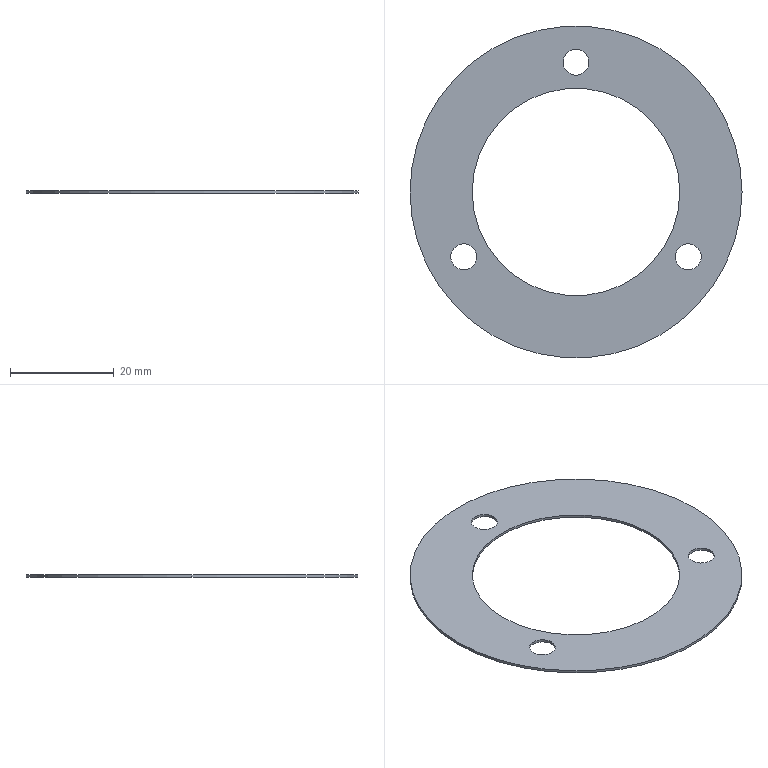Part | SolidWorks | features Extrusion 1, ICE 1 | 1 solid | 12 faces | box 64 x 64 x 0.5 mm | volume 950.724 mm3 | cylinder 10 | plane 2 | commonest cylinder face diameters 5 x6 40 x2 64 x2
STEP:
#1=CARTESIAN_POINT('',(-2.5,25.,0.));
#2=VERTEX_POINT('',#1);
#3=CARTESIAN_POINT('',(2.5,25.,0.));
#4=VERTEX_POINT('',#3);
#5=CARTESIAN_POINT('',(0.,25.,0.));
#6=DIRECTION('',(0.,0.,1.));
#7=DIRECTION('',(1.,0.,0.));
#8=AXIS2_PLACEMENT_3D('',#5,#6,#7);
#9=CIRCLE('',#8,2.5);
#10=EDGE_CURVE('',#2,#4,#9,.T.);
#11=ORIENTED_EDGE('',*,*,#10,.F.);
#12=CARTESIAN_POINT('',(-2.5,25.,0.5));
#13=VERTEX_POINT('',#12);
#14=CARTESIAN_POINT('',(-2.5,25.,0.));
#15=DIRECTION('',(0.,0.,1.));
#16=VECTOR('',#15,1000.);
#17=LINE('',#14,#16);
#18=EDGE_CURVE('',#2,#13,#17,.T.);
#19=ORIENTED_EDGE('',*,*,#18,.T.);
#20=CARTESIAN_POINT('',(2.5,25.,0.5));
#21=VERTEX_POINT('',#20);
#22=CARTESIAN_POINT('',(0.,25.,0.5));
#23=DIRECTION('',(0.,0.,1.));
#24=DIRECTION('',(1.,0.,0.));
#25=AXIS2_PLACEMENT_3D('',#22,#23,#24);
#26=CIRCLE('',#25,2.5);
#27=EDGE_CURVE('',#13,#21,#26,.T.);
#28=ORIENTED_EDGE('',*,*,#27,.T.);
#29=CARTESIAN_POINT('',(2.5,25.,0.));
#30=DIRECTION('',(0.,0.,1.));
#31=VECTOR('',#30,1000.);
#32=LINE('',#29,#31);
#33=EDGE_CURVE('',#4,#21,#32,.T.);
#34=ORIENTED_EDGE('',*,*,#33,.F.);
#35=EDGE_LOOP('',(#11,#19,#28,#34));
#36=FACE_OUTER_BOUND('',#35,.T.);
#37=CARTESIAN_POINT('',(0.,25.,0.));
#38=DIRECTION('',(0.,0.,1.));
#39=DIRECTION('',(1.,0.,0.));
#40=AXIS2_PLACEMENT_3D('',#37,#38,#39);
#41=CYLINDRICAL_SURFACE('',#40,2.5);
#42=ADVANCED_FACE('',(#36),#41,.F.);
#43=CARTESIAN_POINT('',(19.151,-12.5,0.));
#44=VERTEX_POINT('',#43);
#45=CARTESIAN_POINT('',(24.151,-12.5,0.));
#46=VERTEX_POINT('',#45);
#47=CARTESIAN_POINT('',(21.651,-12.5,0.));
#48=DIRECTION('',(0.,0.,1.));
#49=DIRECTION('',(1.,0.,0.));
#50=AXIS2_PLACEMENT_3D('',#47,#48,#49);
#51=CIRCLE('',#50,2.5);
#52=EDGE_CURVE('',#44,#46,#51,.T.);
#53=ORIENTED_EDGE('',*,*,#52,.F.);
#54=CARTESIAN_POINT('',(19.151,-12.5,0.5));
#55=VERTEX_POINT('',#54);
#56=CARTESIAN_POINT('',(19.151,-12.5,0.));
#57=DIRECTION('',(0.,0.,1.));
#58=VECTOR('',#57,1000.);
#59=LINE('',#56,#58);
#60=EDGE_CURVE('',#44,#55,#59,.T.);
#61=ORIENTED_EDGE('',*,*,#60,.T.);
#62=CARTESIAN_POINT('',(24.151,-12.5,0.5));
#63=VERTEX_POINT('',#62);
#64=CARTESIAN_POINT('',(21.651,-12.5,0.5));
#65=DIRECTION('',(0.,0.,1.));
#66=DIRECTION('',(1.,0.,0.));
#67=AXIS2_PLACEMENT_3D('',#64,#65,#66);
#68=CIRCLE('',#67,2.5);
#69=EDGE_CURVE('',#55,#63,#68,.T.);
#70=ORIENTED_EDGE('',*,*,#69,.T.);
#71=CARTESIAN_POINT('',(24.151,-12.5,0.));
#72=DIRECTION('',(0.,0.,1.));
#73=VECTOR('',#72,1000.);
#74=LINE('',#71,#73);
#75=EDGE_CURVE('',#46,#63,#74,.T.);
#76=ORIENTED_EDGE('',*,*,#75,.F.);
#77=EDGE_LOOP('',(#53,#61,#70,#76));
#78=FACE_OUTER_BOUND('',#77,.T.);
#79=CARTESIAN_POINT('',(21.651,-12.5,0.));
#80=DIRECTION('',(0.,0.,1.));
#81=DIRECTION('',(1.,0.,0.));
#82=AXIS2_PLACEMENT_3D('',#79,#80,#81);
#83=CYLINDRICAL_SURFACE('',#82,2.5);
#84=ADVANCED_FACE('',(#78),#83,.F.);
#85=CARTESIAN_POINT('',(-24.151,-12.5,0.));
#86=VERTEX_POINT('',#85);
#87=CARTESIAN_POINT('',(-19.151,-12.5,0.));
#88=VERTEX_POINT('',#87);
#89=CARTESIAN_POINT('',(-21.651,-12.5,0.));
#90=DIRECTION('',(0.,0.,1.));
#91=DIRECTION('',(1.,0.,0.));
#92=AXIS2_PLACEMENT_3D('',#89,#90,#91);
#93=CIRCLE('',#92,2.5);
#94=EDGE_CURVE('',#86,#88,#93,.T.);
#95=ORIENTED_EDGE('',*,*,#94,.F.);
#96=CARTESIAN_POINT('',(-24.151,-12.5,0.5));
#97=VERTEX_POINT('',#96);
#98=CARTESIAN_POINT('',(-24.151,-12.5,0.));
#99=DIRECTION('',(0.,0.,1.));
#100=VECTOR('',#99,1000.);
#101=LINE('',#98,#100);
#102=EDGE_CURVE('',#86,#97,#101,.T.);
#103=ORIENTED_EDGE('',*,*,#102,.T.);
#104=CARTESIAN_POINT('',(-19.151,-12.5,0.5));
#105=VERTEX_POINT('',#104);
#106=CARTESIAN_POINT('',(-21.651,-12.5,0.5));
#107=DIRECTION('',(0.,0.,1.));
#108=DIRECTION('',(1.,0.,0.));
#109=AXIS2_PLACEMENT_3D('',#106,#107,#108);
#110=CIRCLE('',#109,2.5);
#111=EDGE_CURVE('',#97,#105,#110,.T.);
#112=ORIENTED_EDGE('',*,*,#111,.T.);
#113=CARTESIAN_POINT('',(-19.151,-12.5,0.));
#114=DIRECTION('',(0.,0.,1.));
#115=VECTOR('',#114,1000.);
#116=LINE('',#113,#115);
#117=EDGE_CURVE('',#88,#105,#116,.T.);
#118=ORIENTED_EDGE('',*,*,#117,.F.);
#119=EDGE_LOOP('',(#95,#103,#112,#118));
#120=FACE_OUTER_BOUND('',#119,.T.);
#121=CARTESIAN_POINT('',(-21.651,-12.5,0.));
#122=DIRECTION('',(0.,0.,1.));
#123=DIRECTION('',(1.,0.,0.));
#124=AXIS2_PLACEMENT_3D('',#121,#122,#123);
#125=CYLINDRICAL_SURFACE('',#124,2.5);
#126=ADVANCED_FACE('',(#120),#125,.F.);
#127=CARTESIAN_POINT('',(-20.,0.,0.5));
#128=VERTEX_POINT('',#127);
#129=CARTESIAN_POINT('',(20.,0.,0.5));
#130=VERTEX_POINT('',#129);
#131=CARTESIAN_POINT('',(0.,0.,0.5));
#132=DIRECTION('',(0.,0.,1.));
#133=DIRECTION('',(1.,0.,0.));
#134=AXIS2_PLACEMENT_3D('',#131,#132,#133);
#135=CIRCLE('',#134,20.);
#136=EDGE_CURVE('',#128,#130,#135,.T.);
#137=ORIENTED_EDGE('',*,*,#136,.T.);
#138=CARTESIAN_POINT('',(20.,0.,0.));
#139=VERTEX_POINT('',#138);
#140=CARTESIAN_POINT('',(20.,0.,0.5));
#141=DIRECTION('',(0.,0.,-1.));
#142=VECTOR('',#141,1000.);
#143=LINE('',#140,#142);
#144=EDGE_CURVE('',#130,#139,#143,.T.);
#145=ORIENTED_EDGE('',*,*,#144,.T.);
#146=CARTESIAN_POINT('',(-20.,0.,0.));
#147=VERTEX_POINT('',#146);
#148=CARTESIAN_POINT('',(0.,0.,0.));
#149=DIRECTION('',(0.,0.,1.));
#150=DIRECTION('',(1.,0.,0.));
#151=AXIS2_PLACEMENT_3D('',#148,#149,#150);
#152=CIRCLE('',#151,20.);
#153=EDGE_CURVE('',#147,#139,#152,.T.);
#154=ORIENTED_EDGE('',*,*,#153,.F.);
#155=CARTESIAN_POINT('',(-20.,0.,0.5));
#156=DIRECTION('',(0.,0.,-1.));
#157=VECTOR('',#156,1000.);
#158=LINE('',#155,#157);
#159=EDGE_CURVE('',#128,#147,#158,.T.);
#160=ORIENTED_EDGE('',*,*,#159,.F.);
#161=EDGE_LOOP('',(#137,#145,#154,#160));
#162=FACE_OUTER_BOUND('',#161,.T.);
#163=CARTESIAN_POINT('',(0.,0.,0.5));
#164=DIRECTION('',(0.,0.,-1.));
#165=DIRECTION('',(-1.,0.,0.));
#166=AXIS2_PLACEMENT_3D('',#163,#164,#165);
#167=CYLINDRICAL_SURFACE('',#166,20.);
#168=ADVANCED_FACE('',(#162),#167,.F.);
#169=CARTESIAN_POINT('',(32.,0.,0.5));
#170=VERTEX_POINT('',#169);
#171=CARTESIAN_POINT('',(-32.,0.,0.5));
#172=VERTEX_POINT('',#171);
#173=CARTESIAN_POINT('',(0.,0.,0.5));
#174=DIRECTION('',(0.,0.,1.));
#175=DIRECTION('',(1.,0.,0.));
#176=AXIS2_PLACEMENT_3D('',#173,#174,#175);
#177=CIRCLE('',#176,32.);
#178=EDGE_CURVE('',#170,#172,#177,.T.);
#179=ORIENTED_EDGE('',*,*,#178,.F.);
#180=CARTESIAN_POINT('',(32.,0.,0.));
#181=VERTEX_POINT('',#180);
#182=CARTESIAN_POINT('',(32.,0.,0.5));
#183=DIRECTION('',(0.,0.,-1.));
#184=VECTOR('',#183,1000.);
#185=LINE('',#182,#184);
#186=EDGE_CURVE('',#170,#181,#185,.T.);
#187=ORIENTED_EDGE('',*,*,#186,.T.);
#188=CARTESIAN_POINT('',(-32.,0.,0.));
#189=VERTEX_POINT('',#188);
#190=CARTESIAN_POINT('',(0.,0.,0.));
#191=DIRECTION('',(0.,0.,1.));
#192=DIRECTION('',(1.,0.,0.));
#193=AXIS2_PLACEMENT_3D('',#190,#191,#192);
#194=CIRCLE('',#193,32.);
#195=EDGE_CURVE('',#181,#189,#194,.T.);
#196=ORIENTED_EDGE('',*,*,#195,.T.);
#197=CARTESIAN_POINT('',(-32.,0.,0.5));
#198=DIRECTION('',(0.,0.,-1.));
#199=VECTOR('',#198,1000.);
#200=LINE('',#197,#199);
#201=EDGE_CURVE('',#172,#189,#200,.T.);
#202=ORIENTED_EDGE('',*,*,#201,.F.);
#203=EDGE_LOOP('',(#179,#187,#196,#202));
#204=FACE_OUTER_BOUND('',#203,.T.);
#205=CARTESIAN_POINT('',(0.,0.,0.5));
#206=DIRECTION('',(0.,0.,-1.));
#207=DIRECTION('',(-1.,0.,0.));
#208=AXIS2_PLACEMENT_3D('',#205,#206,#207);
#209=CYLINDRICAL_SURFACE('',#208,32.);
#210=ADVANCED_FACE('',(#204),#209,.T.);
#211=CARTESIAN_POINT('',(0.,25.,0.5));
#212=DIRECTION('',(0.,0.,1.));
#213=DIRECTION('',(1.,0.,0.));
#214=AXIS2_PLACEMENT_3D('',#211,#212,#213);
#215=CIRCLE('',#214,2.5);
#216=EDGE_CURVE('',#21,#13,#215,.T.);
#217=ORIENTED_EDGE('',*,*,#216,.F.);
#218=ORIENTED_EDGE('',*,*,#27,.F.);
#219=EDGE_LOOP('',(#217,#218));
#220=FACE_BOUND('',#219,.T.);
#221=CARTESIAN_POINT('',(21.651,-12.5,0.5));
#222=DIRECTION('',(0.,0.,1.));
#223=DIRECTION('',(1.,0.,0.));
#224=AXIS2_PLACEMENT_3D('',#221,#222,#223);
#225=CIRCLE('',#224,2.5);
#226=EDGE_CURVE('',#63,#55,#225,.T.);
#227=ORIENTED_EDGE('',*,*,#226,.F.);
#228=ORIENTED_EDGE('',*,*,#69,.F.);
#229=EDGE_LOOP('',(#227,#228));
#230=FACE_BOUND('',#229,.T.);
#231=CARTESIAN_POINT('',(-21.651,-12.5,0.5));
#232=DIRECTION('',(0.,0.,1.));
#233=DIRECTION('',(1.,0.,0.));
#234=AXIS2_PLACEMENT_3D('',#231,#232,#233);
#235=CIRCLE('',#234,2.5);
#236=EDGE_CURVE('',#105,#97,#235,.T.);
#237=ORIENTED_EDGE('',*,*,#236,.F.);
#238=ORIENTED_EDGE('',*,*,#111,.F.);
#239=EDGE_LOOP('',(#237,#238));
#240=FACE_BOUND('',#239,.T.);
#241=CARTESIAN_POINT('',(0.,0.,0.5));
#242=DIRECTION('',(0.,0.,1.));
#243=DIRECTION('',(1.,0.,0.));
#244=AXIS2_PLACEMENT_3D('',#241,#242,#243);
#245=CIRCLE('',#244,32.);
#246=EDGE_CURVE('',#172,#170,#245,.T.);
#247=ORIENTED_EDGE('',*,*,#246,.T.);
#248=ORIENTED_EDGE('',*,*,#178,.T.);
#249=EDGE_LOOP('',(#247,#248));
#250=FACE_OUTER_BOUND('',#249,.T.);
#251=ORIENTED_EDGE('',*,*,#136,.F.);
#252=CARTESIAN_POINT('',(0.,0.,0.5));
#253=DIRECTION('',(0.,0.,1.));
#254=DIRECTION('',(1.,0.,0.));
#255=AXIS2_PLACEMENT_3D('',#252,#253,#254);
#256=CIRCLE('',#255,20.);
#257=EDGE_CURVE('',#130,#128,#256,.T.);
#258=ORIENTED_EDGE('',*,*,#257,.F.);
#259=EDGE_LOOP('',(#251,#258));
#260=FACE_BOUND('',#259,.T.);
#261=CARTESIAN_POINT('',(0.,0.,0.5));
#262=DIRECTION('',(0.,0.,1.));
#263=DIRECTION('',(1.,0.,0.));
#264=AXIS2_PLACEMENT_3D('',#261,#262,#263);
#265=PLANE('',#264);
#266=ADVANCED_FACE('',(#220,#230,#240,#250,#260),#265,.T.);
#267=CARTESIAN_POINT('',(0.,25.,0.));
#268=DIRECTION('',(0.,0.,1.));
#269=DIRECTION('',(1.,0.,0.));
#270=AXIS2_PLACEMENT_3D('',#267,#268,#269);
#271=CIRCLE('',#270,2.5);
#272=EDGE_CURVE('',#4,#2,#271,.T.);
#273=ORIENTED_EDGE('',*,*,#272,.T.);
#274=ORIENTED_EDGE('',*,*,#10,.T.);
#275=EDGE_LOOP('',(#273,#274));
#276=FACE_BOUND('',#275,.T.);
#277=CARTESIAN_POINT('',(21.651,-12.5,0.));
#278=DIRECTION('',(0.,0.,1.));
#279=DIRECTION('',(1.,0.,0.));
#280=AXIS2_PLACEMENT_3D('',#277,#278,#279);
#281=CIRCLE('',#280,2.5);
#282=EDGE_CURVE('',#46,#44,#281,.T.);
#283=ORIENTED_EDGE('',*,*,#282,.T.);
#284=ORIENTED_EDGE('',*,*,#52,.T.);
#285=EDGE_LOOP('',(#283,#284));
#286=FACE_BOUND('',#285,.T.);
#287=CARTESIAN_POINT('',(-21.651,-12.5,0.));
#288=DIRECTION('',(0.,0.,1.));
#289=DIRECTION('',(1.,0.,0.));
#290=AXIS2_PLACEMENT_3D('',#287,#288,#289);
#291=CIRCLE('',#290,2.5);
#292=EDGE_CURVE('',#88,#86,#291,.T.);
#293=ORIENTED_EDGE('',*,*,#292,.T.);
#294=ORIENTED_EDGE('',*,*,#94,.T.);
#295=EDGE_LOOP('',(#293,#294));
#296=FACE_BOUND('',#295,.T.);
#297=CARTESIAN_POINT('',(0.,0.,0.));
#298=DIRECTION('',(0.,0.,1.));
#299=DIRECTION('',(1.,0.,0.));
#300=AXIS2_PLACEMENT_3D('',#297,#298,#299);
#301=CIRCLE('',#300,32.);
#302=EDGE_CURVE('',#189,#181,#301,.T.);
#303=ORIENTED_EDGE('',*,*,#302,.F.);
#304=ORIENTED_EDGE('',*,*,#195,.F.);
#305=EDGE_LOOP('',(#303,#304));
#306=FACE_OUTER_BOUND('',#305,.T.);
#307=ORIENTED_EDGE('',*,*,#153,.T.);
#308=CARTESIAN_POINT('',(0.,0.,0.));
#309=DIRECTION('',(0.,0.,1.));
#310=DIRECTION('',(1.,0.,0.));
#311=AXIS2_PLACEMENT_3D('',#308,#309,#310);
#312=CIRCLE('',#311,20.);
#313=EDGE_CURVE('',#139,#147,#312,.T.);
#314=ORIENTED_EDGE('',*,*,#313,.T.);
#315=EDGE_LOOP('',(#307,#314));
#316=FACE_BOUND('',#315,.T.);
#317=CARTESIAN_POINT('',(0.,0.,0.));
#318=DIRECTION('',(0.,0.,1.));
#319=DIRECTION('',(1.,0.,0.));
#320=AXIS2_PLACEMENT_3D('',#317,#318,#319);
#321=PLANE('',#320);
#322=ADVANCED_FACE('',(#276,#286,#296,#306,#316),#321,.F.);
#323=ORIENTED_EDGE('',*,*,#186,.F.);
#324=ORIENTED_EDGE('',*,*,#246,.F.);
#325=ORIENTED_EDGE('',*,*,#201,.T.);
#326=ORIENTED_EDGE('',*,*,#302,.T.);
#327=EDGE_LOOP('',(#323,#324,#325,#326));
#328=FACE_OUTER_BOUND('',#327,.T.);
#329=CARTESIAN_POINT('',(0.,0.,0.5));
#330=DIRECTION('',(0.,0.,-1.));
#331=DIRECTION('',(-1.,0.,0.));
#332=AXIS2_PLACEMENT_3D('',#329,#330,#331);
#333=CYLINDRICAL_SURFACE('',#332,32.);
#334=ADVANCED_FACE('',(#328),#333,.T.);
#335=ORIENTED_EDGE('',*,*,#144,.F.);
#336=ORIENTED_EDGE('',*,*,#257,.T.);
#337=ORIENTED_EDGE('',*,*,#159,.T.);
#338=ORIENTED_EDGE('',*,*,#313,.F.);
#339=EDGE_LOOP('',(#335,#336,#337,#338));
#340=FACE_OUTER_BOUND('',#339,.T.);
#341=CARTESIAN_POINT('',(0.,0.,0.5));
#342=DIRECTION('',(0.,0.,-1.));
#343=DIRECTION('',(-1.,0.,0.));
#344=AXIS2_PLACEMENT_3D('',#341,#342,#343);
#345=CYLINDRICAL_SURFACE('',#344,20.);
#346=ADVANCED_FACE('',(#340),#345,.F.);
#347=ORIENTED_EDGE('',*,*,#102,.F.);
#348=ORIENTED_EDGE('',*,*,#292,.F.);
#349=ORIENTED_EDGE('',*,*,#117,.T.);
#350=ORIENTED_EDGE('',*,*,#236,.T.);
#351=EDGE_LOOP('',(#347,#348,#349,#350));
#352=FACE_OUTER_BOUND('',#351,.T.);
#353=CARTESIAN_POINT('',(-21.651,-12.5,0.));
#354=DIRECTION('',(0.,0.,1.));
#355=DIRECTION('',(1.,0.,0.));
#356=AXIS2_PLACEMENT_3D('',#353,#354,#355);
#357=CYLINDRICAL_SURFACE('',#356,2.5);
#358=ADVANCED_FACE('',(#352),#357,.F.);
#359=ORIENTED_EDGE('',*,*,#60,.F.);
#360=ORIENTED_EDGE('',*,*,#282,.F.);
#361=ORIENTED_EDGE('',*,*,#75,.T.);
#362=ORIENTED_EDGE('',*,*,#226,.T.);
#363=EDGE_LOOP('',(#359,#360,#361,#362));
#364=FACE_OUTER_BOUND('',#363,.T.);
#365=CARTESIAN_POINT('',(21.651,-12.5,0.));
#366=DIRECTION('',(0.,0.,1.));
#367=DIRECTION('',(1.,0.,0.));
#368=AXIS2_PLACEMENT_3D('',#365,#366,#367);
#369=CYLINDRICAL_SURFACE('',#368,2.5);
#370=ADVANCED_FACE('',(#364),#369,.F.);
#371=ORIENTED_EDGE('',*,*,#18,.F.);
#372=ORIENTED_EDGE('',*,*,#272,.F.);
#373=ORIENTED_EDGE('',*,*,#33,.T.);
#374=ORIENTED_EDGE('',*,*,#216,.T.);
#375=EDGE_LOOP('',(#371,#372,#373,#374));
#376=FACE_OUTER_BOUND('',#375,.T.);
#377=CARTESIAN_POINT('',(0.,25.,0.));
#378=DIRECTION('',(0.,0.,1.));
#379=DIRECTION('',(1.,0.,0.));
#380=AXIS2_PLACEMENT_3D('',#377,#378,#379);
#381=CYLINDRICAL_SURFACE('',#380,2.5);
#382=ADVANCED_FACE('',(#376),#381,.F.);
#383=CLOSED_SHELL('',(#42,#84,#126,#168,#210,#266,#322,#334,#346,#358,#370,#382));
#384=MANIFOLD_SOLID_BREP('',#383);
#385=CARTESIAN_POINT('',(0.,0.,0.));
#386=DIRECTION('',(0.,0.,1.));
#387=DIRECTION('',(1.,0.,0.));
#388=AXIS2_PLACEMENT_3D('',#385,#386,#387);
#389=(LENGTH_UNIT()NAMED_UNIT(*)SI_UNIT(.MILLI.,.METRE.));
#390=UNCERTAINTY_MEASURE_WITH_UNIT(LENGTH_MEASURE(0.00001),#389,'','');
#391=(NAMED_UNIT(*)PLANE_ANGLE_UNIT()SI_UNIT($,.RADIAN.));
#392=(NAMED_UNIT(*)SI_UNIT($,.STERADIAN.)SOLID_ANGLE_UNIT());
#393=(GEOMETRIC_REPRESENTATION_CONTEXT(3)GLOBAL_UNCERTAINTY_ASSIGNED_CONTEXT((#390))GLOBAL_UNIT_ASSIGNED_CONTEXT((#389,#391,#392))REPRESENTATION_CONTEXT('',''));
#394=ADVANCED_BREP_SHAPE_REPRESENTATION('',(#384,#388),#393);